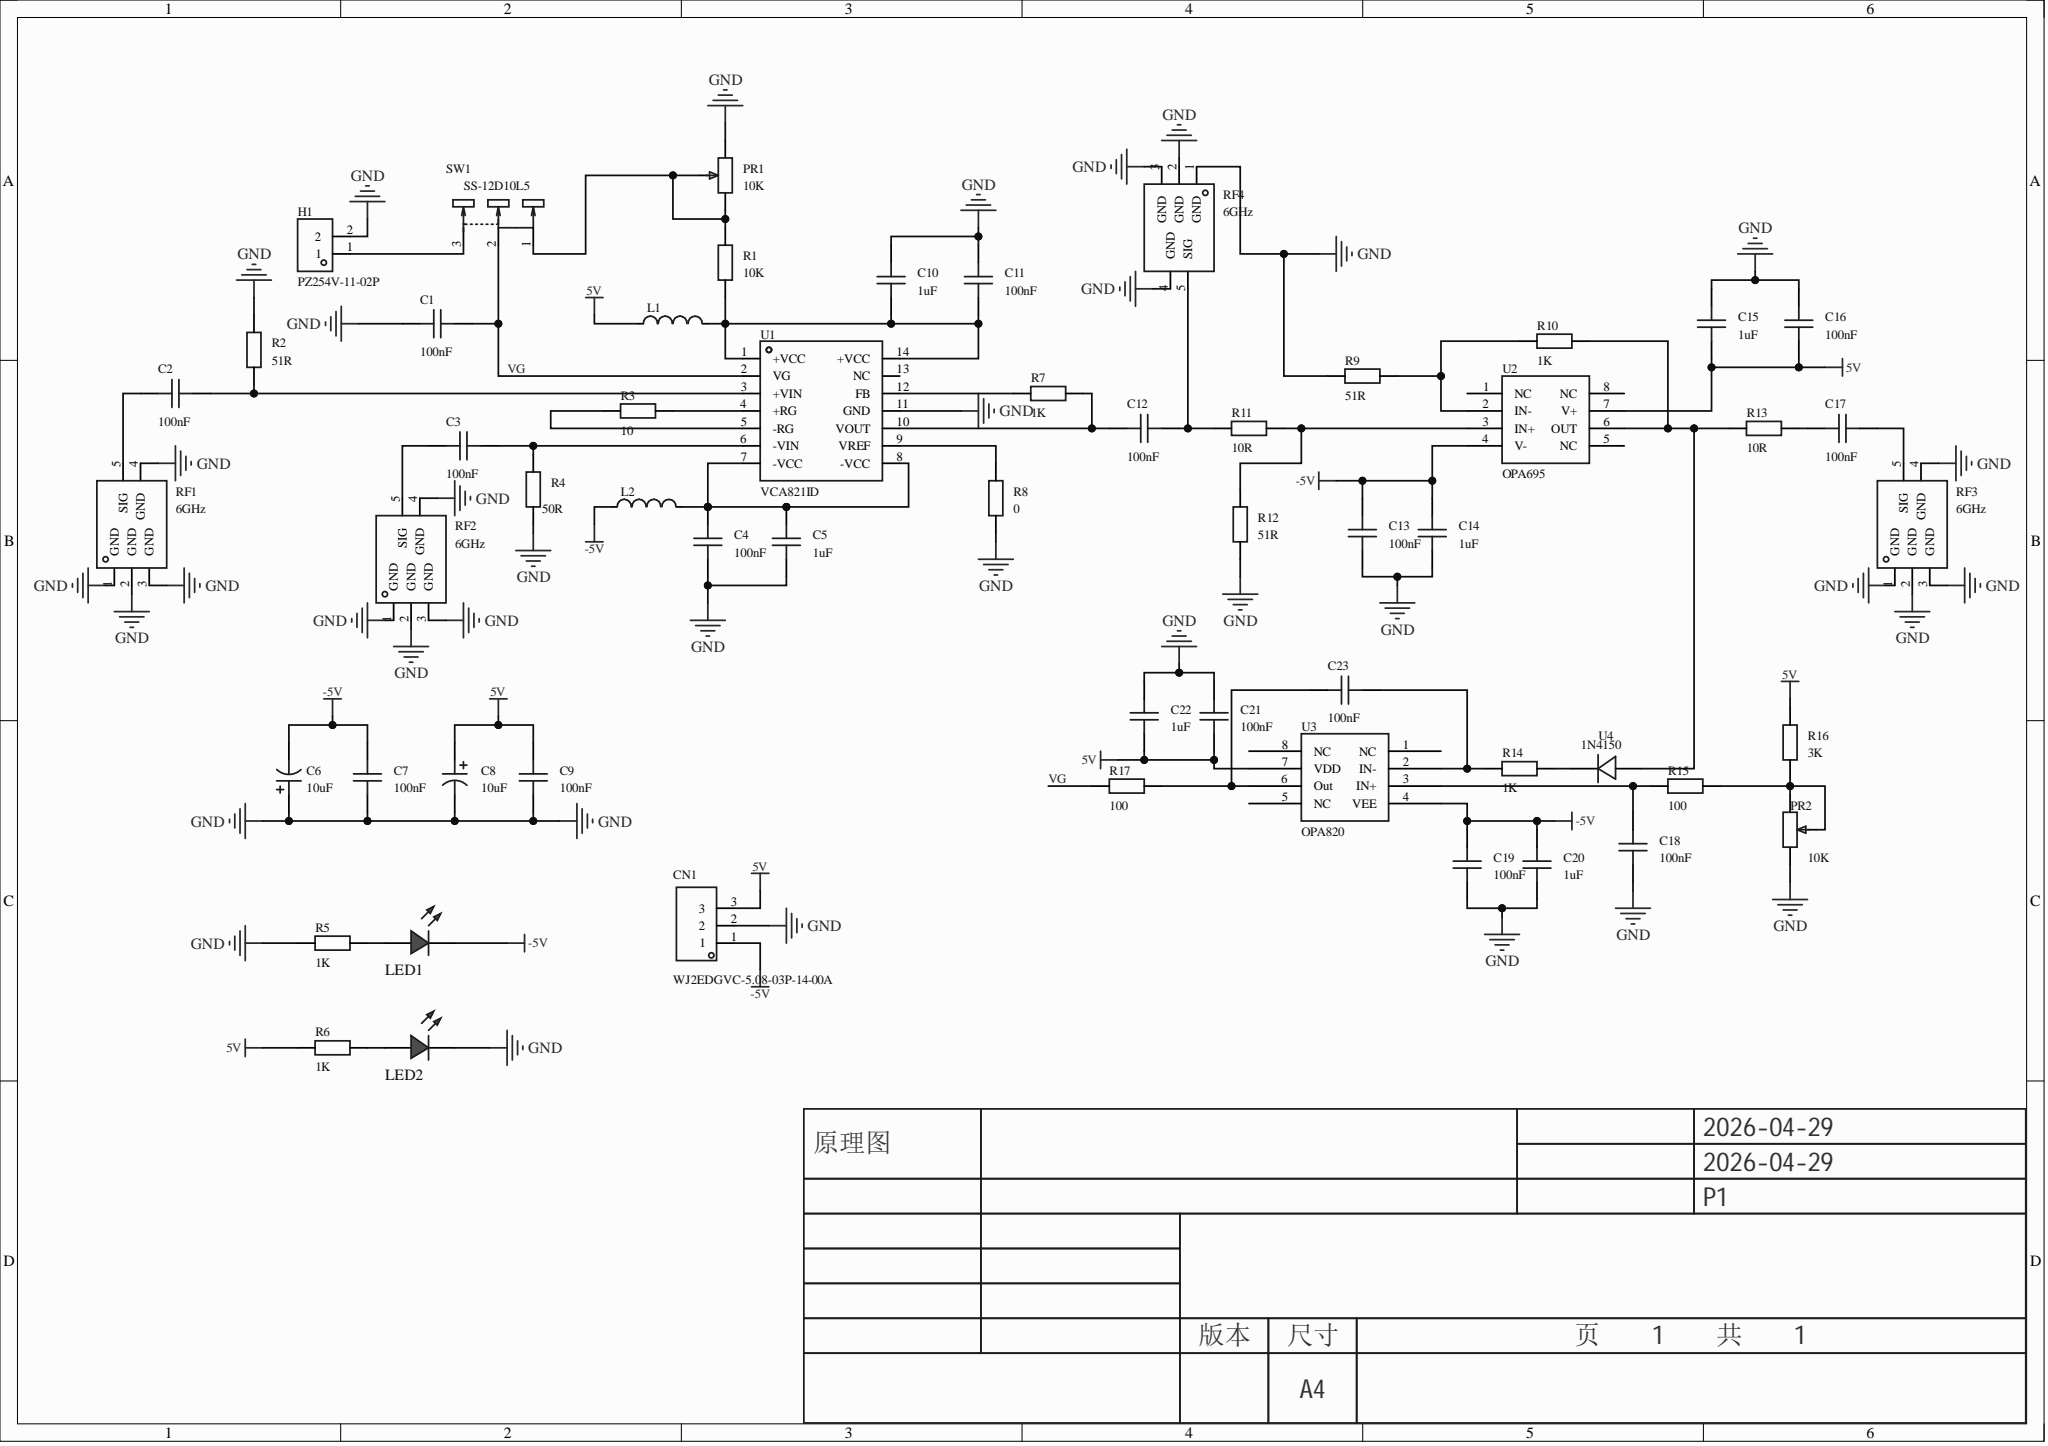Circuit board | Altium Designer | 57 parts | 30 nets
Bill of materials:
Comment,Description,Designator,Footprint,LibRef,Quantity
"100nF","","C1, C2, C3, C4, C7, C9, C11, C12, C13, C16, C17, C18, C19, C21, C23","C0603","CAP_0603, CL10B104KB8NNNC","15"
"1uF","","C5, C10, C14, C15, C20, C22","C0603","CAP_0603, CL10B104KB8NNNC","6"
"10uF","","C6, C8","CAP-TH_BD5.0-P2.00-D0.5-FD-A","ERG50V10M5X11","2"
"WJ2EDGVC-5.08-03P-14-00A","连接器类型:板端/插座-闭口;固定方式:卡扣固定;结构:1x3P;间距:5.08mm;颜色:绿色;安装方式:直插;排数:1;每排PIN数:3;额定电流:10A;额定电压:300V;线规 - AWG:-;线规 - 平方毫米:-;工作温度:-40℃~+105℃;","CN1","CONN-TH_3P-P5.08-WJ2EDGVC-3P","WJ2EDGVC-5.08-03P-14-00A","1"
"PZ254V-11-02P","插针结构:1x2P;间距:2.54mm;行距:-;圆针/方针:方针;安装方式:直插;排数:单排;总PIN位数:2P;额定电流:3A;额定电压:250V;配合针长度:6mm;塑高:2.5mm;端接针长度:3mm;触头材质:黄铜;触头镀层:-;工作温度:-40℃~+105℃;颜色:黑色;","H1","HDR-TH_2P-P2.54-V-M","PZ254V-11-02P","1"
"10uH","","L1, L2","L0603","L_0603","2"
"","","LED1, LED2","LED_0603","LED_0603-R","2"
"10K","","PR1, PR2","R_3386P","R_3386P","2"
"10K","","R1","R0603","Res_0603","1"
"51R","","R2, R9, R12","R0603","Res_0603","3"
"10","","R3","R0603","Res_0603","1"
"50R","","R4","R0603","Res_0603","1"
"1K","","R5, R6, R7, R10, R14","R0603","Res_0603","5"
"0","","R8","R0603","Res_0603","1"
"10R","","R11, R13","R0603","Res_0603","2"
"100","","R15, R17","R0603","Res_0603","2"
"3K","","R16","R0603","Res_0603","1"
"6GHz","","RF1, RF2, RF3, RF4","SMA-SMD_BWSMA-KE-P001","SMA-KHD9A","4"
"SS-12D10L5","电路结构:单刀双掷;安装方式:直插;开关颜色:黑色;额定电流:3A;额定电压:125V;工作寿命:1万次;","SW1","SW-TH_SS-12D10L5","SS-12D10L5","1"
"VCA821ID","放大器类型:VGA;通道数:单路;增益:32dB;带宽(-3db):710MHz;压摆率(SR):2500V/us;轨到轨:-;输出电流:90mA;","U1","SOIC-14_L8.7-W3.9-P1.27-LS6.0-BL","VCA821ID","1"
"OPA695","","U2","SOIC-8","OPA695","1"
"OPA820","","U3","SOP8","OPA820","1"
"1N4150","二极管配置:1个独立式;正向压降(Vf):1V@200mA;直流反向耐压(Vr):50V;整流电流:200mA;反向恢复时间(Trr):4ns;","U4","SOD-123_L2.7-W1.6-LS3.7-RD-1","1N4150W-E3-18","1"
Netlist (Protel format):
[
C1
C0603
100nF



]
[
C2
C0603
100nF



]
[
C3
C0603
100nF



]
[
C4
C0603
100nF



]
[
C5
C0603
1uF



]
[
C6
CAP-TH_BD5.0-P2.00-D0.5-FD-A
10uF



]
[
C7
C0603
100nF



]
[
C8
CAP-TH_BD5.0-P2.00-D0.5-FD-A
10uF



]
[
C9
C0603
100nF



]
[
C10
C0603
1uF



]
[
C11
C0603
100nF



]
[
C12
C0603
100nF



]
[
C13
C0603
100nF



]
[
C14
C0603
1uF



]
[
C15
C0603
1uF



]
[
C16
C0603
100nF



]
[
C17
C0603
100nF



]
[
C18
C0603
100nF



]
[
C19
C0603
100nF



]
[
C20
C0603
1uF



]
[
C21
C0603
100nF



]
[
C22
C0603
1uF



]
[
C23
C0603
100nF



]
[
CN1
CONN-TH_3P-P5.08-WJ2EDGVC-3P
WJ2EDGVC-5.08-03P-14-00A



]
[
H1
HDR-TH_2P-P2.54-V-M
PZ254V-11-02P



]
[
L1
L0603
10uH



]
[
L2
L0603
10uH



]
[
LED1
LED_0603




]
[
LED2
LED_0603




]
[
PR1
R_3386P
10K



]
[
PR2
R_3386P
10K



]
[
R1
R0603
10K



]
[
R2
R0603
51R



]
[
R3
R0603
10



]
[
R4
R0603
50R



]
[
R5
R0603
1K



]
[
R6
R0603
1K



]
[
R7
R0603
1K



]
[
R8
R0603
0



]
[
R9
R0603
51R



]
[
R10
R0603
1K



]
[
R11
R0603
10R



]
[
R12
R0603
51R



]
[
R13
R0603
10R



]
[
R14
R0603
1K



]
[
R15
R0603
100



]
[
R16
R0603
3K



]
[
R17
R0603
100



]
[
RF1
SMA-SMD_BWSMA-KE-P001
6GHz



]
[
RF2
SMA-SMD_BWSMA-KE-P001
6GHz



]
[
RF3
SMA-SMD_BWSMA-KE-P001
6GHz



]
[
RF4
SMA-SMD_BWSMA-KE-P001
6GHz



]
[
SW1
SW-TH_SS-12D10L5
SS-12D10L5



]
[
U1
SOIC-14_L8.7-W3.9-P1.27-LS6.0-BL
VCA821ID



]
[
U2
SOIC-8
OPA695



]
[
U3
SOP8
OPA820



]
[
U4
SOD-123_L2.7-W1.6-LS3.7-RD-1
1N4150



]
(
VG
C1-2
R17-1
SW1-2
U1-2
)
(
NetR14_2
R14-2
U4-1
)
(
NetR11_2
R11-2
R12-2
U2-3
)
(
NetR10_2
R10-2
R13-1
U2-6
U4-2
)
(
NetR9_2
R9-2
R10-1
U2-2
)
(
NetR8_2
R8-2
U1-9
)
(
NetR7_1
R7-1
U1-12
)
(
NetR3_2
R3-2
U1-4
)
(
NetR3_1
R3-1
U1-5
)
(
NetPR2_2
PR2-2
PR2-3
R15-2
R16-1
)
(
NetPR1_2
PR1-2
PR1-3
R1-2
SW1-1
)
(
NetLED2_2
LED2-2
R6-2
)
(
NetLED1_2
LED1-2
R5-2
)
(
NetH1_1
H1-1
SW1-3
)
(
NetC23_2
C23-2
R17-2
U3-6
)
(
NetC23_1
C23-1
R14-1
U3-2
)
(
NetC18_2
C18-2
R15-1
U3-3
)
(
NetC17_2
C17-2
RF3-5
)
(
NetC17_1
C17-1
R13-2
)
(
NetC12_2
C12-2
R11-1
RF4-5
)
(
NetC12_1
C12-1
R7-2
U1-10
)
(
NetC10_1
C10-1
C11-1
L1-2
R1-1
U1-1
U1-14
)
(
NetC4_1
C4-1
C5-2
L2-2
U1-7
U1-8
)
(
NetC3_2
C3-2
R4-2
U1-6
)
(
NetC3_1
C3-1
RF2-5
)
(
NetC2_2
C2-2
R2-1
U1-3
)
(
NetC2_1
C2-1
RF1-5
)
(
GND
C1-1
C4-2
C5-1
C6-1
C7-1
C8-2
C9-1
C10-2
C11-2
C13-1
C14-1
C15-2
C16-2
C18-1
C19-1
C20-1
C21-2
C22-2
CN1-2
H1-2
LED2-1
PR1-1
PR2-1
R2-2
R4-1
R5-1
R8-1
R9-1
R12-1
RF1-1
RF1-2
RF1-3
RF1-4
RF2-1
RF2-2
RF2-3
RF2-4
RF3-1
RF3-2
RF3-3
RF3-4
RF4-1
RF4-2
RF4-3
RF4-4
U1-11
)
(
-5V
C6-2
C7-2
C13-2
C14-2
C19-2
C20-2
CN1-1
L2-1
LED1-1
U2-4
U3-4
)
(
5V
C8-1
C9-2
C15-1
C16-1
C21-1
C22-1
CN1-3
L1-1
R6-1
R16-2
U2-7
U3-7
)